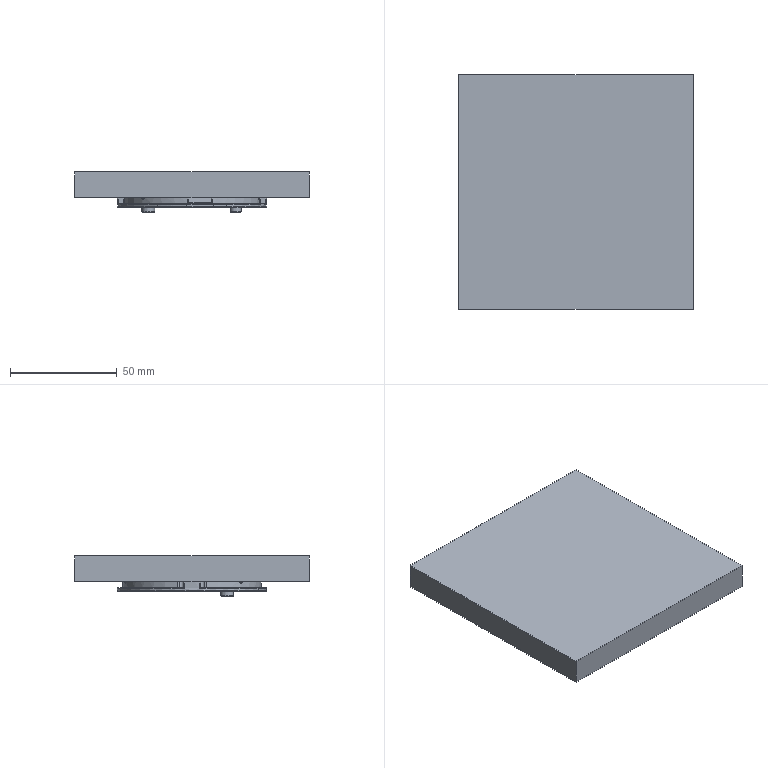NC program | NX | posted with a generic post | part box 110 x 110 x 18.8 mm
Lines 804 to 1647 of 8004:
(FLOOR_WALL_1_COPY , TOOL : D3)
N1576 T17 M6
N1578 G54
N1580 G17 G0 G90 X-3.034 Y37.677 S9500 M3
N1582 G43 Z30. H17
N1584 Z-0.8
N1586 G94 G1 Z-2.3 F1000.
N1588 X-2.184 Y36.375
N1590 G3 X-1.917 Y36.239 R0.3
N1592 G2 X32.711 Y-15.739 R36.29
N1594 X2.584 Y-36.21 R36.308
N1596 G1 X2.209 Y-36.187
N1598 X-10.181 Y-34.784
N1600 X-10.582 Y-34.726
N1602 G2 X-23.328 Y27.813 R36.303
N1604 X-1.917 Y36.239 R36.198
N1606 G1 X-1.835 Y34.742
N1608 G2 X29.78 Y-18.005 R34.791
N1610 X2.559 Y-34.706 R34.8
N1612 G1 X2.341 Y-34.692
N1614 X-9.99 Y-33.296
N1616 X-10.235 Y-33.261
N1618 G2 X-22.363 Y26.663 R34.8
N1620 X-1.835 Y34.742 R34.702
N1622 G1 X-1.754 Y33.244
N1624 G2 X28.496 Y-17.229 R33.291
N1626 X2.473 Y-33.197 R33.253
N1628 G1 X-9.888 Y-31.795
N1630 G2 X-21.399 Y25.514 R33.297
N1632 X-1.754 Y33.244 R33.205
N1634 G1 X-1.672 Y31.746
N1636 G2 X27.212 Y-16.453 R31.791
N1638 X2.531 Y-31.694 R31.782
N1640 G1 X-9.55 Y-30.327
N1642 G2 X-20.435 Y24.364 R31.795
N1644 X-1.672 Y31.746 R31.709
N1646 G1 X-1.591 Y30.248
N1648 G2 X25.928 Y-15.676 R30.291
N1650 G1 X25.545 Y-16.277
N1652 G3 X21.369 Y-21.475 R-5.05
N1654 G1 X21.317 Y-21.179
N1656 G2 X15.821 Y-17.317 R4.75
N1658 X21.317 Y-21.179 R-4.75
N1660 G1 X21.369 Y-21.475
N1662 G2 X2.542 Y-30.186 R30.221
N1664 G1 X-9.225 Y-28.854
N1666 G2 X-22.043 Y-20.78 R30.125
N1668 G3 X-25.011 Y-17.096 R-4.55
N1670 G1 X-24.713 Y-17.056
N1672 G2 X-21.056 Y-12.287 R4.25
N1674 X-24.713 Y-17.056 R-4.25
N1676 G1 X-25.011 Y-17.096
N1678 G2 X-1.591 Y30.248 R30.287
N1680 G1 X-1.509 Y28.751
N1682 G2 X25.839 Y-12.705 R28.785
N1684 G3 X17.931 Y-22.525 R-6.55
N1686 G2 X2.554 Y-28.678 R28.617
N1688 G1 X-8.899 Y-27.381
N1690 G2 X-18.376 Y-22.165 R28.42
N1692 G3 X-25.58 Y-13.214 R-6.05
N1694 G2 X-1.509 Y28.751 R28.782
N1696 G1 X-1.428 Y27.253
N1698 G2 X25.359 Y-10.082 R27.281
N1700 G3 X15.273 Y-22.622 R8.05
N1702 G2 X2.565 Y-27.169 R27.141
N1704 G1 X-8.574 Y-25.908
N1706 G2 X-15.696 Y-22.325 R26.594
N1708 G3 X-25.164 Y-10.563 R7.55
N1710 G2 X-1.428 Y27.253 R27.28
N1712 G1 X-1.346 Y25.755
N1714 G2 X24.568 Y-7.86 R25.786
N1716 G3 X12.926 Y-22.317 R9.55
N1718 G2 X2.577 Y-25.661 R25.478
N1720 G1 X-8.248 Y-24.436
N1722 G2 X-13.362 Y-22.063 R24.911
N1724 G3 X-24.408 Y-8.337 R9.05
N1726 G2 X-1.346 Y25.755 R25.782
N1728 G1 X-1.265 Y24.257
N1730 G2 X23.568 Y-5.884 R24.282
N1732 G3 X10.787 Y-21.768 R11.05
N1734 G1 X10.677 Y-21.826
N1736 G2 X2.588 Y-24.153 R24.085
N1738 G1 X-7.923 Y-22.963
N1740 X-8.245 Y-22.855
N1742 X-9.324 Y-22.437
N1744 X-10.383 Y-21.967
N1746 X-11.232 Y-21.54
N1748 G3 X-23.444 Y-6.369 R10.55
N1750 G2 X-1.265 Y24.257 R24.284
N1752 G1 X-1.183 Y22.759
N1754 G2 X22.419 Y-4.098 R22.78
N1756 G3 X8.795 Y-21.027 R12.55
N1758 G2 X2.6 Y-22.645 R22.401
N1760 G1 X-7.597 Y-21.49
N1762 X-8.749 Y-21.051
N1764 X-9.254 Y-20.827
N1766 G3 X-22.323 Y-4.589 R12.05
N1768 G2 X-1.183 Y22.759 R22.778
N1770 G1 X-1.102 Y21.262
N1772 G2 X21.152 Y-2.465 R21.287
N1774 G3 X6.927 Y-20.132 R14.05
N1776 G2 X2.605 Y-21.136 R20.631
N1778 G1 X-7.263 Y-20.019
N1780 X-7.401 Y-19.965
N1782 G3 X-21.085 Y-2.963 R13.55
N1784 G2 X-1.102 Y21.262 R21.28
N1786 G1 X-1.02 Y19.764
N1788 G2 X19.767 Y-0.967 R19.779
N1790 G3 X5.17 Y-19.109 R15.55
N1792 G1 X4.254 Y-19.333
N1794 X3.328 Y-19.514
N1796 X2.58 Y-19.623
N1798 X-5.611 Y-18.696
N1800 G3 X-19.739 Y-1.469 R15.05
N1802 G2 X-1.02 Y19.764 R19.782
N1804 G1 X-0.939 Y18.266
N1806 G2 X18.289 Y0.406 R18.283
N1808 G3 X3.512 Y-17.95 R17.05
N1810 G1 X3.076 Y-18.035
N1812 X2.556 Y-18.111
N1814 X-3.973 Y-17.372
N1816 G3 X-18.29 Y-0.098 R16.55
N1818 G2 X-0.939 Y18.266 R18.277
N1820 G1 X-0.857 Y16.768
N1822 G2 X16.708 Y1.658 R16.778
N1824 G3 X1.95 Y-16.5 R18.55
N1826 G1 Y-16.533
N1828 X-2.456 Y-16.034
N1830 G3 X-16.753 Y1.157 R18.05
N1832 G2 X-0.857 Y16.768 R16.781
N1834 G1 X-0.776 Y15.271
N1836 G2 X15.034 Y2.791 R15.279
N1838 G3 X0.517 Y-14.861 R20.05
N1840 G1 X-1.034 Y-14.685
N1842 G3 X-15.119 Y2.295 R19.55
N1844 G2 X-0.776 Y15.271 R15.28
N1846 G1 X-0.694 Y13.773
N1848 G2 X13.258 Y3.797 R13.778
N1850 G3 X-0.26 Y-10.718 R21.55
N1852 X-13.388 Y3.312 R21.05
N1854 G2 X-0.694 Y13.773 R13.778
N1856 G1 X-0.612 Y12.275
N1858 G2 X11.37 Y4.665 R12.275
N1860 G3 X-0.278 Y-6.521 R23.05
N1862 X-11.554 Y4.2 R22.55
N1864 G2 X-0.612 Y12.275 R12.284
N1866 G1 X-0.531 Y10.777
N1868 G2 X9.356 Y5.375 R10.774
N1870 G3 X-0.296 Y-3.453 R24.55
N1872 X-9.595 Y4.936 R24.05
N1874 G2 X-0.531 Y10.777 R10.772
N1876 G1 X-0.449 Y9.279
N1878 G2 X7.185 Y5.89 R9.274
N1880 G3 X-0.315 Y-0.836 R26.05
N1882 X-7.495 Y5.493 R25.55
N1884 G2 X-0.449 Y9.279 R9.278
N1886 G1 X-0.368 Y7.782
N1888 G2 X4.798 Y6.137 R7.758
N1890 G3 X-0.333 Y1.528 R27.55
N1892 X-5.196 Y5.804 R27.05
N1894 G2 X-0.368 Y7.782 R7.758
N1896 G1 X-0.286 Y6.284
N1898 G2 X2.057 Y5.944 R6.201
N1900 G3 X-0.351 Y3.727 R29.05
N1902 X-2.589 Y5.733 R28.55
N1904 G2 X-0.286 Y6.284 R6.211
N1906 G3 X-0.035 Y6.448 R0.3
N1908 G1 Z-0.8
N1910 G0 Z30.
N1912 X-26.15 Y-17.568
N1914 Z-0.8
N1916 G1 Z-2.3
N1918 X-24.75 Y-16.76
N1920 G3 X-24.6 Y-16.5 R0.3
N1922 G2 X-20.5 Y-12.4 R4.1
N1924 X-24.6 Y-16.5 R-4.1
N1926 G3 X-24.75 Y-16.24 R0.3
N1928 G1 X-26.15 Y-15.432
N1930 Z-0.8
N1932 G0 Z30.
N1934 X26.657 Y-15.428
N1936 Z-0.8
N1938 G1 Z-2.3
N1940 X25.25 Y-16.24
N1942 G3 X25.1 Y-16.5 R0.3
N1944 G2 X20.5 Y-21.1 R4.6
N1946 X25.1 Y-16.5 R-4.6
N1948 G3 X25.25 Y-16.76 R0.3
N1950 G1 X26.657 Y-17.572
N1952 Z-0.8
N1954 G0 Z30.
(ZLEVEL_PROFILE_1_COPY_1_COPY , TOOL : D3)
N1956 X-12.5 Y-11.879
N1958 Z-2.8
N1960 G1 Y-8.728 Z-2.965
N1962 X-12.545 Y-8.746 Z-2.968
N1964 X-12.773 Y-8.881 Z-2.982
N1966 X-13.244 Y-9.28 Z-3.014
N1968 X-13.639 Y-9.756 Z-3.046
N1970 X-13.943 Y-10.293 Z-3.079
N1972 X-14.149 Y-10.876 Z-3.111
N1974 X-14.25 Y-11.485 Z-3.143
N1976 Y-16. Z-3.38
N1978 X-12.5 Z-3.472
N1980 Y-8.728 Z-3.853
N1982 X-12.545 Y-8.746 Z-3.855
N1984 X-12.773 Y-8.881 Z-3.869
N1986 X-13.244 Y-9.28 Z-3.902
N1988 X-13.639 Y-9.756 Z-3.934
N1990 X-13.943 Y-10.293 Z-3.966
N1992 X-14.149 Y-10.876 Z-3.999
N1994 X-14.25 Y-11.485 Z-4.031
N1996 Y-16. Z-4.268
N1998 X-12.5 Z-4.359
N2000 Y-12.364 Z-4.55
N2002 Y-8.728
N2004 X-12.545 Y-8.746
N2006 G3 X-14.25 Y-11.75 R3.5
N2008 G1 Y-16.
N2010 X-12.5
N2012 Y-12.364
N2014 Y-8.945 Z-4.617
N2016 Y-8.774 Z-4.62
N2018 Y-8.729 Z-4.621
N2020 X-12.527 Y-8.745 Z-4.622
N2022 X-12.731 Y-8.869 Z-4.627
N2024 X-12.828 Y-8.943 Z-4.629
N2026 X-12.924 Y-9.018 Z-4.632
N2028 X-13.02 Y-9.093 Z-4.634
N2030 X-13.111 Y-9.175 Z-4.637
N2032 X-13.197 Y-9.26 Z-4.639
N2034 X-13.283 Y-9.347 Z-4.641
N2036 X-13.37 Y-9.433 Z-4.644
N2038 X-13.445 Y-9.529 Z-4.646
N2040 X-13.52 Y-9.625 Z-4.649
N2042 X-13.595 Y-9.721 Z-4.651
N2044 X-13.664 Y-9.822 Z-4.653
N2046 X-13.727 Y-9.926 Z-4.656
N2048 X-13.79 Y-10.03 Z-4.658
N2050 X-13.852 Y-10.135 Z-4.661
N2052 X-13.902 Y-10.246 Z-4.663
N2054 X-13.951 Y-10.358 Z-4.665
N2056 X-14.002 Y-10.469 Z-4.668
N2058 X-14.043 Y-10.584 Z-4.67
N2060 X-14.08 Y-10.7 Z-4.673
N2062 X-14.116 Y-10.816 Z-4.675
N2064 X-14.149 Y-10.933 Z-4.677
N2066 X-14.172 Y-11.053 Z-4.68
N2068 X-14.194 Y-11.173 Z-4.682
N2070 X-14.216 Y-11.293 Z-4.685
N2072 X-14.227 Y-11.414 Z-4.687
N2074 X-14.234 Y-11.536 Z-4.689
N2076 X-14.242 Y-11.658 Z-4.692
N2078 X-14.25 Y-11.78 Z-4.694
N2080 Y-16. Z-4.777
N2082 X-13.097 Z-4.8
N2084 X-12.5
N2086 Y-12.364
N2088 Y-8.945 Z-4.867
N2090 Y-8.774 Z-4.87
N2092 Y-8.729 Z-4.871
N2094 X-12.527 Y-8.745 Z-4.872
N2096 X-12.731 Y-8.869 Z-4.877
N2098 X-12.828 Y-8.943 Z-4.879
N2100 X-12.924 Y-9.018 Z-4.882
N2102 X-13.02 Y-9.093 Z-4.884
N2104 X-13.111 Y-9.175 Z-4.887
N2106 X-13.197 Y-9.26 Z-4.889
N2108 X-13.283 Y-9.347 Z-4.891
N2110 X-13.37 Y-9.433 Z-4.894
N2112 X-13.445 Y-9.529 Z-4.896
N2114 X-13.52 Y-9.625 Z-4.899
N2116 X-13.595 Y-9.721 Z-4.901
N2118 X-13.664 Y-9.822 Z-4.903
N2120 X-13.727 Y-9.926 Z-4.906
N2122 X-13.79 Y-10.03 Z-4.908
N2124 X-13.852 Y-10.135 Z-4.911
N2126 X-13.902 Y-10.246 Z-4.913
N2128 X-13.951 Y-10.358 Z-4.915
N2130 X-14.002 Y-10.469 Z-4.918
N2132 X-14.043 Y-10.584 Z-4.92
N2134 X-14.08 Y-10.7 Z-4.923
N2136 X-14.116 Y-10.816 Z-4.925
N2138 X-14.149 Y-10.933 Z-4.927
N2140 X-14.172 Y-11.053 Z-4.93
N2142 X-14.194 Y-11.173 Z-4.932
N2144 X-14.216 Y-11.293 Z-4.935
N2146 X-14.227 Y-11.414 Z-4.937
N2148 X-14.234 Y-11.536 Z-4.939
N2150 X-14.242 Y-11.658 Z-4.942
N2152 X-14.25 Y-11.78 Z-4.944
N2154 Y-16. Z-5.027
N2156 X-13.097 Z-5.05
N2158 X-12.5
N2160 Y-12.364
N2162 Y-8.945 Z-5.117
N2164 Y-8.775 Z-5.12
N2166 Y-8.729 Z-5.121
N2168 X-12.527 Y-8.745 Z-5.122
N2170 X-12.731 Y-8.869 Z-5.127
N2172 X-12.828 Y-8.943 Z-5.129
N2174 X-12.924 Y-9.018 Z-5.132
N2176 X-13.02 Y-9.093 Z-5.134
N2178 X-13.111 Y-9.175 Z-5.137
N2180 X-13.197 Y-9.26 Z-5.139
N2182 X-13.283 Y-9.347 Z-5.141
N2184 X-13.37 Y-9.433 Z-5.144
N2186 X-13.445 Y-9.529 Z-5.146
N2188 X-13.52 Y-9.625 Z-5.149
N2190 X-13.595 Y-9.721 Z-5.151
N2192 X-13.664 Y-9.822 Z-5.153
N2194 X-13.727 Y-9.926 Z-5.156
N2196 X-13.79 Y-10.03 Z-5.158
N2198 X-13.852 Y-10.135 Z-5.161
N2200 X-13.902 Y-10.246 Z-5.163
N2202 X-13.951 Y-10.358 Z-5.165
N2204 X-14.002 Y-10.469 Z-5.168
N2206 X-14.043 Y-10.584 Z-5.17
N2208 X-14.08 Y-10.7 Z-5.173
N2210 X-14.116 Y-10.816 Z-5.175
N2212 X-14.149 Y-10.933 Z-5.177
N2214 X-14.172 Y-11.053 Z-5.18
N2216 X-14.194 Y-11.173 Z-5.182
N2218 X-14.216 Y-11.293 Z-5.185
N2220 X-14.227 Y-11.414 Z-5.187
N2222 X-14.234 Y-11.536 Z-5.189
N2224 X-14.242 Y-11.658 Z-5.192
N2226 X-14.25 Y-11.78 Z-5.194
N2228 Y-16. Z-5.277
N2230 X-13.097 Z-5.3
N2232 X-12.5
N2234 Y-12.364
N2236 Y-8.945 Z-5.367
N2238 Y-8.775 Z-5.37
N2240 Y-8.729 Z-5.371
N2242 X-12.527 Y-8.745 Z-5.372
N2244 X-12.731 Y-8.869 Z-5.377
N2246 X-12.828 Y-8.943 Z-5.379
N2248 X-12.924 Y-9.018 Z-5.382
N2250 X-13.02 Y-9.093 Z-5.384
N2252 X-13.111 Y-9.175 Z-5.387
N2254 X-13.197 Y-9.26 Z-5.389
N2256 X-13.283 Y-9.347 Z-5.391
N2258 X-13.37 Y-9.433 Z-5.394
N2260 X-13.445 Y-9.529 Z-5.396
N2262 X-13.52 Y-9.625 Z-5.399
N2264 X-13.595 Y-9.721 Z-5.401
N2266 X-13.664 Y-9.822 Z-5.403
N2268 X-13.727 Y-9.926 Z-5.406
N2270 X-13.79 Y-10.03 Z-5.408
N2272 X-13.852 Y-10.135 Z-5.411
N2274 X-13.902 Y-10.247 Z-5.413
N2276 X-13.951 Y-10.358 Z-5.415
N2278 X-14.002 Y-10.469 Z-5.418
N2280 X-14.043 Y-10.584 Z-5.42
N2282 X-14.08 Y-10.7 Z-5.423
N2284 X-14.116 Y-10.816 Z-5.425
N2286 X-14.149 Y-10.934 Z-5.427
N2288 X-14.172 Y-11.053 Z-5.43
N2290 X-14.194 Y-11.173 Z-5.432
N2292 X-14.216 Y-11.293 Z-5.435
N2294 X-14.227 Y-11.415 Z-5.437
N2296 X-14.234 Y-11.536 Z-5.439
N2298 X-14.242 Y-11.658 Z-5.442
N2300 X-14.25 Y-11.78 Z-5.444
N2302 Y-16. Z-5.527
N2304 X-13.097 Z-5.55
N2306 X-12.5
N2308 Y-12.364
N2310 Y-8.945 Z-5.617
N2312 Y-8.775 Z-5.62
N2314 Y-8.729 Z-5.621
N2316 X-12.527 Y-8.745 Z-5.622
N2318 X-12.731 Y-8.869 Z-5.627
N2320 X-12.828 Y-8.943 Z-5.629
N2322 X-12.924 Y-9.019 Z-5.632
N2324 X-13.02 Y-9.093 Z-5.634
N2326 X-13.111 Y-9.175 Z-5.637
N2328 X-13.197 Y-9.26 Z-5.639
N2330 X-13.283 Y-9.347 Z-5.641
N2332 X-13.37 Y-9.433 Z-5.644
N2334 X-13.445 Y-9.529 Z-5.646
N2336 X-13.52 Y-9.625 Z-5.649
N2338 X-13.595 Y-9.721 Z-5.651
N2340 X-13.664 Y-9.822 Z-5.653
N2342 X-13.727 Y-9.926 Z-5.656
N2344 X-13.79 Y-10.03 Z-5.658
N2346 X-13.852 Y-10.136 Z-5.661
N2348 X-13.902 Y-10.247 Z-5.663
N2350 X-13.951 Y-10.358 Z-5.665
N2352 X-14.002 Y-10.469 Z-5.668
N2354 X-14.043 Y-10.584 Z-5.67
N2356 X-14.079 Y-10.7 Z-5.673
N2358 X-14.116 Y-10.816 Z-5.675
N2360 X-14.149 Y-10.934 Z-5.677
N2362 X-14.172 Y-11.053 Z-5.68
N2364 X-14.194 Y-11.173 Z-5.682
N2366 X-14.216 Y-11.293 Z-5.685
N2368 X-14.227 Y-11.415 Z-5.687
N2370 X-14.234 Y-11.536 Z-5.689
N2372 X-14.242 Y-11.658 Z-5.692
N2374 X-14.25 Y-11.78 Z-5.694
N2376 Y-16. Z-5.777
N2378 X-13.097 Z-5.8
N2380 X-12.5
N2382 Y-12.364
N2384 Y-8.945 Z-5.867
N2386 Y-8.775 Z-5.87
N2388 Y-8.729 Z-5.871
N2390 X-12.527 Y-8.745 Z-5.872
N2392 X-12.731 Y-8.869 Z-5.877
N2394 X-12.828 Y-8.943 Z-5.879
N2396 X-12.924 Y-9.019 Z-5.882
N2398 X-13.02 Y-9.093 Z-5.884
N2400 X-13.111 Y-9.175 Z-5.887
N2402 X-13.197 Y-9.26 Z-5.889
N2404 X-13.283 Y-9.347 Z-5.891
N2406 X-13.37 Y-9.433 Z-5.894
N2408 X-13.445 Y-9.529 Z-5.896
N2410 X-13.52 Y-9.625 Z-5.899
N2412 X-13.595 Y-9.721 Z-5.901
N2414 X-13.664 Y-9.822 Z-5.903
N2416 X-13.727 Y-9.926 Z-5.906
N2418 X-13.79 Y-10.03 Z-5.908
N2420 X-13.852 Y-10.136 Z-5.911
N2422 X-13.902 Y-10.247 Z-5.913
N2424 X-13.951 Y-10.358 Z-5.915
N2426 X-14.002 Y-10.469 Z-5.918
N2428 X-14.043 Y-10.584 Z-5.92
N2430 X-14.079 Y-10.7 Z-5.923
N2432 X-14.116 Y-10.816 Z-5.925
N2434 X-14.149 Y-10.934 Z-5.927
N2436 X-14.172 Y-11.053 Z-5.93
N2438 X-14.194 Y-11.173 Z-5.932
N2440 X-14.216 Y-11.293 Z-5.935
N2442 X-14.227 Y-11.415 Z-5.937
N2444 X-14.234 Y-11.536 Z-5.939
N2446 X-14.242 Y-11.658 Z-5.942
N2448 X-14.25 Y-11.78 Z-5.944
N2450 Y-16. Z-6.027
N2452 X-13.097 Z-6.05
N2454 X-12.5
N2456 Y-12.364
N2458 Y-8.945 Z-6.117
N2460 Y-8.775 Z-6.12
N2462 Y-8.729 Z-6.121
N2464 X-12.527 Y-8.745 Z-6.122
N2466 X-12.731 Y-8.869 Z-6.127
N2468 X-12.828 Y-8.943 Z-6.129
N2470 X-12.924 Y-9.019 Z-6.132
N2472 X-13.02 Y-9.093 Z-6.134
N2474 X-13.111 Y-9.175 Z-6.137
N2476 X-13.197 Y-9.26 Z-6.139
N2478 X-13.283 Y-9.347 Z-6.141
N2480 X-13.37 Y-9.433 Z-6.144
N2482 X-13.445 Y-9.529 Z-6.146
N2484 X-13.52 Y-9.625 Z-6.149
N2486 X-13.595 Y-9.721 Z-6.151
N2488 X-13.664 Y-9.822 Z-6.153
N2490 X-13.727 Y-9.926 Z-6.156
N2492 X-13.79 Y-10.03 Z-6.158
N2494 X-13.852 Y-10.136 Z-6.161
N2496 X-13.902 Y-10.247 Z-6.163
N2498 X-13.951 Y-10.358 Z-6.165
N2500 X-14.002 Y-10.469 Z-6.168
N2502 X-14.043 Y-10.584 Z-6.17
N2504 X-14.079 Y-10.7 Z-6.173
N2506 X-14.116 Y-10.816 Z-6.175
N2508 X-14.149 Y-10.934 Z-6.177
N2510 X-14.172 Y-11.053 Z-6.18
N2512 X-14.194 Y-11.173 Z-6.182
N2514 X-14.216 Y-11.293 Z-6.185
N2516 X-14.227 Y-11.415 Z-6.187
N2518 X-14.234 Y-11.536 Z-6.189
N2520 X-14.242 Y-11.658 Z-6.192
N2522 X-14.25 Y-11.78 Z-6.194
N2524 Y-16. Z-6.277
N2526 X-13.097 Z-6.3
N2528 X-12.5
N2530 Y-12.364
N2532 Y-8.945 Z-6.367
N2534 Y-8.775 Z-6.37
N2536 Y-8.728 Z-6.371
N2538 X-12.527 Y-8.745 Z-6.372
N2540 X-12.731 Y-8.869 Z-6.377
N2542 X-12.828 Y-8.943 Z-6.379
N2544 X-12.924 Y-9.019 Z-6.382
N2546 X-13.02 Y-9.093 Z-6.384
N2548 X-13.111 Y-9.175 Z-6.387
N2550 X-13.197 Y-9.26 Z-6.389
N2552 X-13.283 Y-9.347 Z-6.391
N2554 X-13.37 Y-9.433 Z-6.394
N2556 X-13.445 Y-9.529 Z-6.396
N2558 X-13.52 Y-9.625 Z-6.399
N2560 X-13.595 Y-9.721 Z-6.401
N2562 X-13.664 Y-9.822 Z-6.403
N2564 X-13.727 Y-9.926 Z-6.406
N2566 X-13.79 Y-10.03 Z-6.408
N2568 X-13.852 Y-10.136 Z-6.411
N2570 X-13.902 Y-10.247 Z-6.413
N2572 X-13.951 Y-10.358 Z-6.415
N2574 X-14.002 Y-10.469 Z-6.418
N2576 X-14.043 Y-10.584 Z-6.42
N2578 X-14.079 Y-10.7 Z-6.423
N2580 X-14.116 Y-10.816 Z-6.425
N2582 X-14.149 Y-10.934 Z-6.427
N2584 X-14.172 Y-11.053 Z-6.43
N2586 X-14.194 Y-11.173 Z-6.432
N2588 X-14.216 Y-11.293 Z-6.435
N2590 X-14.227 Y-11.415 Z-6.437
N2592 X-14.234 Y-11.536 Z-6.439
N2594 X-14.242 Y-11.658 Z-6.442
N2596 X-14.25 Y-11.78 Z-6.444
N2598 Y-16. Z-6.527
N2600 X-13.097 Z-6.55
N2602 X-12.5
N2604 Y-12.364
N2606 Y-8.945 Z-6.617
N2608 Y-8.775 Z-6.62
N2610 Y-8.729 Z-6.621
N2612 X-12.527 Y-8.745 Z-6.622
N2614 X-12.731 Y-8.869 Z-6.627
N2616 X-12.828 Y-8.943 Z-6.629
N2618 X-12.924 Y-9.019 Z-6.632
N2620 X-13.02 Y-9.093 Z-6.634
N2622 X-13.111 Y-9.175 Z-6.637
N2624 X-13.197 Y-9.26 Z-6.639
N2626 X-13.283 Y-9.347 Z-6.641
N2628 X-13.37 Y-9.433 Z-6.644
N2630 X-13.445 Y-9.529 Z-6.646
N2632 X-13.52 Y-9.625 Z-6.649
N2634 X-13.595 Y-9.721 Z-6.651
N2636 X-13.664 Y-9.822 Z-6.653
N2638 X-13.727 Y-9.926 Z-6.656
N2640 X-13.79 Y-10.03 Z-6.658
N2642 X-13.852 Y-10.136 Z-6.661
N2644 X-13.902 Y-10.247 Z-6.663
N2646 X-13.951 Y-10.358 Z-6.665
N2648 X-14.002 Y-10.469 Z-6.668
N2650 X-14.043 Y-10.584 Z-6.67
N2652 X-14.079 Y-10.7 Z-6.673
N2654 X-14.116 Y-10.816 Z-6.675
N2656 X-14.15 Y-10.933 Z-6.677
N2658 X-14.172 Y-11.054 Z-6.68
N2660 X-14.194 Y-11.173 Z-6.682
N2662 X-14.216 Y-11.293 Z-6.685
N2664 X-14.227 Y-11.415 Z-6.687
N2666 X-14.234 Y-11.536 Z-6.689
N2668 X-14.242 Y-11.658 Z-6.692
N2670 X-14.25 Y-11.78 Z-6.694
N2672 Y-16. Z-6.777
N2674 X-13.097 Z-6.8
N2676 X-12.5
N2678 Y-12.364
N2680 Y-8.945 Z-6.867
N2682 Y-8.775 Z-6.87
N2684 Y-8.729 Z-6.871
N2686 X-12.527 Y-8.745 Z-6.872
N2688 X-12.731 Y-8.869 Z-6.877
N2690 X-12.828 Y-8.943 Z-6.879
N2692 X-12.924 Y-9.019 Z-6.882
N2694 X-13.02 Y-9.093 Z-6.884
N2696 X-13.111 Y-9.175 Z-6.887
N2698 X-13.197 Y-9.26 Z-6.889
N2700 X-13.283 Y-9.347 Z-6.891
N2702 X-13.37 Y-9.433 Z-6.894
N2704 X-13.445 Y-9.529 Z-6.896
N2706 X-13.52 Y-9.625 Z-6.899
N2708 X-13.595 Y-9.721 Z-6.901
N2710 X-13.664 Y-9.822 Z-6.903
N2712 X-13.727 Y-9.926 Z-6.906
N2714 X-13.79 Y-10.03 Z-6.908
N2716 X-13.852 Y-10.136 Z-6.911
N2718 X-13.902 Y-10.247 Z-6.913
N2720 X-13.951 Y-10.358 Z-6.915
N2722 X-14.002 Y-10.469 Z-6.918
N2724 X-14.043 Y-10.584 Z-6.92
N2726 X-14.079 Y-10.7 Z-6.923
N2728 X-14.116 Y-10.816 Z-6.925
N2730 X-14.15 Y-10.933 Z-6.927
N2732 X-14.172 Y-11.054 Z-6.93
N2734 X-14.194 Y-11.173 Z-6.932
N2736 X-14.216 Y-11.293 Z-6.935
N2738 X-14.227 Y-11.415 Z-6.937
N2740 X-14.234 Y-11.536 Z-6.939
N2742 X-14.242 Y-11.658 Z-6.942
N2744 X-14.25 Y-11.78 Z-6.944
N2746 Y-16. Z-7.027
N2748 X-13.097 Z-7.05
N2750 X-12.5
N2752 Y-12.364
N2754 Y-8.945 Z-7.117
N2756 Y-8.775 Z-7.12
N2758 Y-8.729 Z-7.121
N2760 X-12.527 Y-8.745 Z-7.122
N2762 X-12.731 Y-8.869 Z-7.127
N2764 X-12.828 Y-8.943 Z-7.129
N2766 X-12.924 Y-9.019 Z-7.132
N2768 X-13.02 Y-9.094 Z-7.134
N2770 X-13.111 Y-9.175 Z-7.137
N2772 X-13.197 Y-9.261 Z-7.139
N2774 X-13.283 Y-9.347 Z-7.141
N2776 X-13.37 Y-9.433 Z-7.144
N2778 X-13.445 Y-9.529 Z-7.146
N2780 X-13.52 Y-9.625 Z-7.149
N2782 X-13.595 Y-9.721 Z-7.151
N2784 X-13.664 Y-9.822 Z-7.153
N2786 X-13.727 Y-9.926 Z-7.156
N2788 X-13.79 Y-10.031 Z-7.158
N2790 X-13.852 Y-10.136 Z-7.161
N2792 X-13.902 Y-10.247 Z-7.163
N2794 X-13.951 Y-10.358 Z-7.165
N2796 X-14.002 Y-10.469 Z-7.168
N2798 X-14.043 Y-10.584 Z-7.17
N2800 X-14.079 Y-10.7 Z-7.173
N2802 X-14.116 Y-10.816 Z-7.175
N2804 X-14.15 Y-10.934 Z-7.177
N2806 X-14.172 Y-11.054 Z-7.18
N2808 X-14.194 Y-11.173 Z-7.182
N2810 X-14.216 Y-11.293 Z-7.185
N2812 X-14.227 Y-11.415 Z-7.187
N2814 X-14.234 Y-11.536 Z-7.189
N2816 X-14.242 Y-11.658 Z-7.192
N2818 X-14.25 Y-11.78 Z-7.194
N2820 Y-16. Z-7.277
N2822 X-13.097 Z-7.3
N2824 X-12.5
N2826 Y-12.364
N2828 Y-8.945 Z-7.367
N2830 Y-8.775 Z-7.37
N2832 Y-8.729 Z-7.371
N2834 X-12.527 Y-8.745 Z-7.372
N2836 X-12.731 Y-8.869 Z-7.377
N2838 X-12.828 Y-8.943 Z-7.379
N2840 X-12.924 Y-9.019 Z-7.382
N2842 X-13.02 Y-9.094 Z-7.384
N2844 X-13.111 Y-9.175 Z-7.387
N2846 X-13.197 Y-9.261 Z-7.389
N2848 X-13.283 Y-9.347 Z-7.391
N2850 X-13.37 Y-9.433 Z-7.394
N2852 X-13.445 Y-9.529 Z-7.396
N2854 X-13.52 Y-9.625 Z-7.399
N2856 X-13.595 Y-9.721 Z-7.401
N2858 X-13.664 Y-9.822 Z-7.403
N2860 X-13.727 Y-9.926 Z-7.406
N2862 X-13.79 Y-10.031 Z-7.408
N2864 X-13.852 Y-10.136 Z-7.411
N2866 X-13.902 Y-10.247 Z-7.413
N2868 X-13.951 Y-10.358 Z-7.415
N2870 X-14.002 Y-10.469 Z-7.418
N2872 X-14.043 Y-10.584 Z-7.42
N2874 X-14.079 Y-10.7 Z-7.423
N2876 X-14.116 Y-10.816 Z-7.425
N2878 X-14.15 Y-10.934 Z-7.427
N2880 X-14.172 Y-11.054 Z-7.43
N2882 X-14.193 Y-11.173 Z-7.432
N2884 X-14.216 Y-11.293 Z-7.435
N2886 X-14.227 Y-11.415 Z-7.437
N2888 X-14.234 Y-11.536 Z-7.439
N2890 X-14.242 Y-11.658 Z-7.442
N2892 X-14.25 Y-11.78 Z-7.444
N2894 Y-16. Z-7.527
N2896 X-13.097 Z-7.55
N2898 X-12.5
N2900 Y-12.364
N2902 Y-8.945 Z-7.617
N2904 Y-8.775 Z-7.62
N2906 Y-8.729 Z-7.621
N2908 X-12.527 Y-8.745 Z-7.622
N2910 X-12.731 Y-8.869 Z-7.627
N2912 X-12.828 Y-8.943 Z-7.629
N2914 X-12.924 Y-9.019 Z-7.632
N2916 X-13.02 Y-9.094 Z-7.634
N2918 X-13.111 Y-9.175 Z-7.637
N2920 X-13.197 Y-9.261 Z-7.639
N2922 X-13.283 Y-9.347 Z-7.641
N2924 X-13.37 Y-9.433 Z-7.644
N2926 X-13.445 Y-9.529 Z-7.646
N2928 X-13.52 Y-9.625 Z-7.649
N2930 X-13.595 Y-9.721 Z-7.651
N2932 X-13.663 Y-9.822 Z-7.653
N2934 X-13.727 Y-9.926 Z-7.656
N2936 X-13.79 Y-10.031 Z-7.658
N2938 X-13.852 Y-10.136 Z-7.661
N2940 X-13.902 Y-10.247 Z-7.663
N2942 X-13.951 Y-10.358 Z-7.665
N2944 X-14.002 Y-10.469 Z-7.668
N2946 X-14.043 Y-10.584 Z-7.67
N2948 X-14.079 Y-10.7 Z-7.673
N2950 X-14.116 Y-10.816 Z-7.675
N2952 X-14.15 Y-10.934 Z-7.677
N2954 X-14.172 Y-11.054 Z-7.68
N2956 X-14.193 Y-11.173 Z-7.682
N2958 X-14.216 Y-11.293 Z-7.685
N2960 X-14.227 Y-11.415 Z-7.687
N2962 X-14.234 Y-11.536 Z-7.689
N2964 X-14.242 Y-11.658 Z-7.692
N2966 X-14.25 Y-11.78 Z-7.694
N2968 Y-16. Z-7.777
N2970 X-13.097 Z-7.8
N2972 X-12.5
N2974 Y-12.364
N2976 Y-8.945 Z-7.867
N2978 Y-8.775 Z-7.87
N2980 Y-8.729 Z-7.871
N2982 X-12.527 Y-8.745 Z-7.872
N2984 X-12.731 Y-8.869 Z-7.877
N2986 X-12.828 Y-8.943 Z-7.879
N2988 X-12.924 Y-9.019 Z-7.882
N2990 X-13.02 Y-9.094 Z-7.884
N2992 X-13.111 Y-9.175 Z-7.887
N2994 X-13.197 Y-9.261 Z-7.889
N2996 X-13.283 Y-9.347 Z-7.891
N2998 X-13.369 Y-9.433 Z-7.894
N3000 X-13.445 Y-9.529 Z-7.896
N3002 X-13.52 Y-9.625 Z-7.899
N3004 X-13.595 Y-9.721 Z-7.901
N3006 X-13.664 Y-9.822 Z-7.903
N3008 X-13.727 Y-9.926 Z-7.906
N3010 X-13.79 Y-10.031 Z-7.908
N3012 X-13.852 Y-10.136 Z-7.911
N3014 X-13.902 Y-10.247 Z-7.913
N3016 X-13.951 Y-10.358 Z-7.915
N3018 X-14.002 Y-10.469 Z-7.918
N3020 X-14.043 Y-10.584 Z-7.92
N3022 X-14.079 Y-10.7 Z-7.923
N3024 X-14.116 Y-10.816 Z-7.925
N3026 X-14.15 Y-10.934 Z-7.927
N3028 X-14.172 Y-11.054 Z-7.93
N3030 X-14.193 Y-11.173 Z-7.932
N3032 X-14.216 Y-11.293 Z-7.935
N3034 X-14.227 Y-11.415 Z-7.937
N3036 X-14.234 Y-11.536 Z-7.939
N3038 X-14.242 Y-11.658 Z-7.942
N3040 X-14.25 Y-11.78 Z-7.944
N3042 Y-16. Z-8.027
N3044 X-13.097 Z-8.05
N3046 X-12.5
N3048 Y-12.364
N3050 Y-8.945 Z-8.117
N3052 Y-8.775 Z-8.12
N3054 Y-8.729 Z-8.121
N3056 X-12.527 Y-8.745 Z-8.122
N3058 X-12.731 Y-8.869 Z-8.127
N3060 X-12.828 Y-8.943 Z-8.129
N3062 X-12.924 Y-9.019 Z-8.132
N3064 X-13.02 Y-9.094 Z-8.134
N3066 X-13.111 Y-9.175 Z-8.137
N3068 X-13.197 Y-9.261 Z-8.139
N3070 X-13.283 Y-9.347 Z-8.141
N3072 X-13.369 Y-9.433 Z-8.144
N3074 X-13.445 Y-9.529 Z-8.146
N3076 X-13.52 Y-9.625 Z-8.149
N3078 X-13.595 Y-9.721 Z-8.151
N3080 X-13.664 Y-9.822 Z-8.153
N3082 X-13.727 Y-9.926 Z-8.156
N3084 X-13.79 Y-10.031 Z-8.158
N3086 X-13.852 Y-10.136 Z-8.161
N3088 X-13.902 Y-10.247 Z-8.163
N3090 X-13.951 Y-10.358 Z-8.165
N3092 X-14.002 Y-10.469 Z-8.168
N3094 X-14.043 Y-10.584 Z-8.17
N3096 X-14.079 Y-10.7 Z-8.173
N3098 X-14.116 Y-10.816 Z-8.175
N3100 X-14.15 Y-10.934 Z-8.177
N3102 X-14.172 Y-11.054 Z-8.18
N3104 X-14.193 Y-11.174 Z-8.182
N3106 X-14.216 Y-11.293 Z-8.185
N3108 X-14.227 Y-11.415 Z-8.187
N3110 X-14.234 Y-11.536 Z-8.189
N3112 X-14.242 Y-11.658 Z-8.192
N3114 X-14.25 Y-11.78 Z-8.194
N3116 Y-16. Z-8.277
N3118 X-13.097 Z-8.3
N3120 X-12.5
N3122 Y-12.364
N3124 Y-8.945 Z-8.367
N3126 Y-8.775 Z-8.37
N3128 Y-8.729 Z-8.371
N3130 X-12.527 Y-8.745 Z-8.372
N3132 X-12.595 Y-8.786 Z-8.374
N3134 X-12.731 Y-8.869 Z-8.377
N3136 X-12.828 Y-8.943 Z-8.379
N3138 X-12.924 Y-9.019 Z-8.382
N3140 X-13.02 Y-9.094 Z-8.384
N3142 X-13.111 Y-9.175 Z-8.387
N3144 X-13.197 Y-9.261 Z-8.389
N3146 X-13.283 Y-9.347 Z-8.391
N3148 X-13.369 Y-9.433 Z-8.394
N3150 X-13.445 Y-9.529 Z-8.396
N3152 X-13.52 Y-9.625 Z-8.399
N3154 X-13.595 Y-9.721 Z-8.401
N3156 X-13.664 Y-9.822 Z-8.403
N3158 X-13.727 Y-9.926 Z-8.406
N3160 X-13.79 Y-10.031 Z-8.408
N3162 X-13.852 Y-10.136 Z-8.411
N3164 X-13.902 Y-10.247 Z-8.413
N3166 X-13.951 Y-10.358 Z-8.415
N3168 X-14.002 Y-10.469 Z-8.418
N3170 X-14.043 Y-10.584 Z-8.42
N3172 X-14.079 Y-10.7 Z-8.423
N3174 X-14.116 Y-10.817 Z-8.425
N3176 X-14.15 Y-10.934 Z-8.427
N3178 X-14.172 Y-11.054 Z-8.43
N3180 X-14.193 Y-11.174 Z-8.432
N3182 X-14.216 Y-11.293 Z-8.435
N3184 X-14.227 Y-11.415 Z-8.437
N3186 X-14.234 Y-11.536 Z-8.439
N3188 X-14.242 Y-11.658 Z-8.442
N3190 X-14.25 Y-11.78 Z-8.444
N3192 Y-16. Z-8.527
N3194 X-13.097 Z-8.55
N3196 X-12.5
N3198 Y-12.364
N3200 Y-8.945 Z-8.617
N3202 Y-8.775 Z-8.62
N3204 Y-8.729 Z-8.621
N3206 X-12.527 Y-8.745 Z-8.622
N3208 X-12.595 Y-8.786 Z-8.623
N3210 X-12.731 Y-8.869 Z-8.627
N3212 X-12.828 Y-8.943 Z-8.629
N3214 X-12.924 Y-9.019 Z-8.632
N3216 X-13.02 Y-9.094 Z-8.634
N3218 X-13.111 Y-9.175 Z-8.637
N3220 X-13.197 Y-9.261 Z-8.639
N3222 X-13.283 Y-9.347 Z-8.641
N3224 X-13.37 Y-9.433 Z-8.644
N3226 X-13.445 Y-9.53 Z-8.646
N3228 X-13.52 Y-9.625 Z-8.649
N3230 X-13.595 Y-9.721 Z-8.651
N3232 X-13.664 Y-9.822 Z-8.653
N3234 X-13.727 Y-9.926 Z-8.656
N3236 X-13.79 Y-10.031 Z-8.658
N3238 X-13.852 Y-10.136 Z-8.661
N3240 X-13.902 Y-10.247 Z-8.663
N3242 X-13.951 Y-10.358 Z-8.665
N3244 X-14.002 Y-10.469 Z-8.668
N3246 X-14.043 Y-10.584 Z-8.67
N3248 X-14.079 Y-10.7 Z-8.673
N3250 X-14.116 Y-10.817 Z-8.675